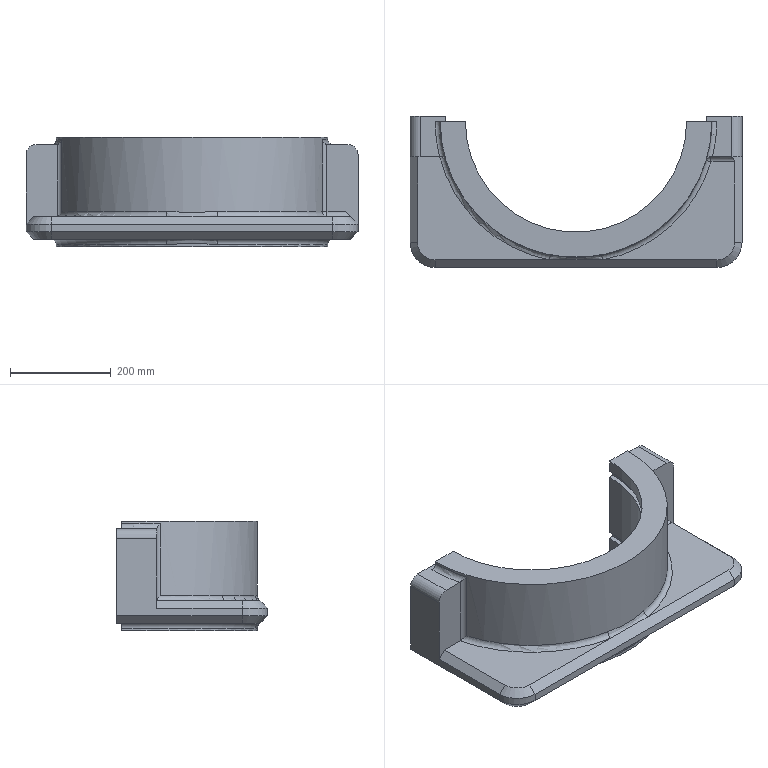Part | SolidWorks | features Fillet 3, ICE 2, MirrorPattern 2, 3DProfileFeature 1, Chamfer 1, Extrusion 1, HoleWzd 1, RevCut 1 | 1 solid | 72 faces | box 660 x 300 x 218 mm | volume 12799321 mm3 | plane 29 | cylinder 22 | cone 12 | torus 6 | spline 2 | sphere 1 | commonest cylinder face diameters 26.5 x8 20 x3 440 x3 40 x2 100 x2 458 x2